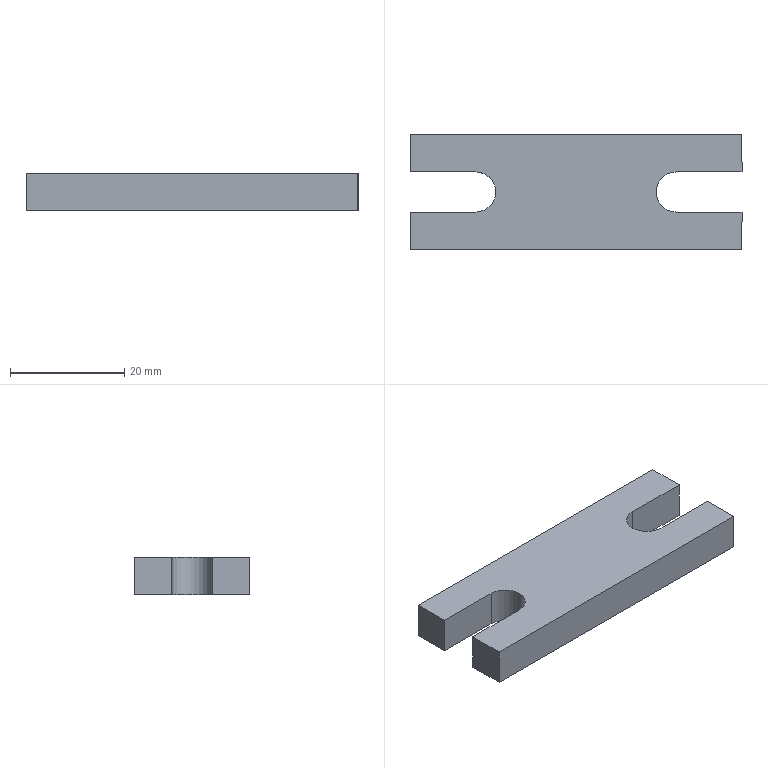Part | STEP file | 601-07-0071 | 1 solid | 15 faces | box 58 x 20 x 6.5 mm | volume 6243 mm3 | plane 12 | cylinder 3 | commonest cylinder face diameters 7 x3
STEP:
#1=CARTESIAN_POINT('',(0.,0.,0.));
#2=DIRECTION('',(0.,0.,1.));
#3=DIRECTION('',(1.,0.,0.));
#4=AXIS2_PLACEMENT_3D('',#1,#2,#3);
#5=CARTESIAN_POINT('',(-11.5,13.5,6.5));
#6=VERTEX_POINT('',#5);
#7=CARTESIAN_POINT('',(-11.5,13.5,0.));
#8=VERTEX_POINT('',#7);
#9=CARTESIAN_POINT('',(-11.5,13.5,6.5));
#10=DIRECTION('',(0.,0.,-1.));
#11=VECTOR('',#10,1.);
#12=LINE('',#9,#11);
#13=CARTESIAN_POINT('',(-11.5,10.,6.5));
#14=DIRECTION('',(0.,0.,-1.));
#15=DIRECTION('',(-1.,0.,0.));
#16=AXIS2_PLACEMENT_3D('',#13,#14,#15);
#17=CYLINDRICAL_SURFACE('',#16,3.5);
#18=CARTESIAN_POINT('',(1.571,0.));
#19=DIRECTION('',(0.,1.));
#20=VECTOR('',#19,1.);
#21=LINE('',#18,#20);
#22=(GEOMETRIC_REPRESENTATION_CONTEXT(2)PARAMETRIC_REPRESENTATION_CONTEXT()REPRESENTATION_CONTEXT('',''));
#23=DEFINITIONAL_REPRESENTATION('',(#21),#22);
#24=PCURVE('',#17,#23);
#25=CARTESIAN_POINT('',(-11.5,13.5,6.5));
#26=DIRECTION('',(0.,1.,0.));
#27=DIRECTION('',(0.,0.,1.));
#28=AXIS2_PLACEMENT_3D('',#25,#26,#27);
#29=PLANE('',#28);
#30=CARTESIAN_POINT('',(0.,0.));
#31=DIRECTION('',(-1.,0.));
#32=VECTOR('',#31,1.);
#33=LINE('',#30,#32);
#34=(GEOMETRIC_REPRESENTATION_CONTEXT(2)PARAMETRIC_REPRESENTATION_CONTEXT()REPRESENTATION_CONTEXT('',''));
#35=DEFINITIONAL_REPRESENTATION('',(#33),#34);
#36=PCURVE('',#29,#35);
#37=SURFACE_CURVE('',#12,(#24,#36),.PCURVE_S1.);
#38=EDGE_CURVE('',#6,#8,#37,.T.);
#39=ORIENTED_EDGE('',*,*,#38,.T.);
#40=CARTESIAN_POINT('',(-15.,10.,0.));
#41=VERTEX_POINT('',#40);
#42=CARTESIAN_POINT('',(-11.5,10.,0.));
#43=DIRECTION('',(0.,0.,-1.));
#44=DIRECTION('',(-1.,0.,0.));
#45=AXIS2_PLACEMENT_3D('',#42,#43,#44);
#46=CIRCLE('',#45,3.5);
#47=CARTESIAN_POINT('',(0.,6.5));
#48=DIRECTION('',(1.,0.));
#49=VECTOR('',#48,1.);
#50=LINE('',#47,#49);
#51=(GEOMETRIC_REPRESENTATION_CONTEXT(2)PARAMETRIC_REPRESENTATION_CONTEXT()REPRESENTATION_CONTEXT('',''));
#52=DEFINITIONAL_REPRESENTATION('',(#50),#51);
#53=PCURVE('',#17,#52);
#54=CARTESIAN_POINT('',(-11.5,10.,0.));
#55=DIRECTION('',(0.,0.,-1.));
#56=DIRECTION('',(-1.,0.,0.));
#57=AXIS2_PLACEMENT_3D('',#54,#55,#56);
#58=PLANE('',#57);
#59=CARTESIAN_POINT('',(0.,0.));
#60=DIRECTION('',(1.,0.));
#61=AXIS2_PLACEMENT_2D('',#59,#60);
#62=CIRCLE('',#61,3.5);
#63=(GEOMETRIC_REPRESENTATION_CONTEXT(2)PARAMETRIC_REPRESENTATION_CONTEXT()REPRESENTATION_CONTEXT('',''));
#64=DEFINITIONAL_REPRESENTATION('',(#62),#63);
#65=PCURVE('',#58,#64);
#66=SURFACE_CURVE('',#46,(#53,#65),.PCURVE_S1.);
#67=EDGE_CURVE('',#41,#8,#66,.T.);
#68=ORIENTED_EDGE('',*,*,#67,.F.);
#69=CARTESIAN_POINT('',(-15.,10.,6.5));
#70=VERTEX_POINT('',#69);
#71=CARTESIAN_POINT('',(-15.,10.,6.5));
#72=DIRECTION('',(0.,0.,-1.));
#73=VECTOR('',#72,1.);
#74=LINE('',#71,#73);
#75=CARTESIAN_POINT('',(0.,0.));
#76=DIRECTION('',(0.,1.));
#77=VECTOR('',#76,1.);
#78=LINE('',#75,#77);
#79=(GEOMETRIC_REPRESENTATION_CONTEXT(2)PARAMETRIC_REPRESENTATION_CONTEXT()REPRESENTATION_CONTEXT('',''));
#80=DEFINITIONAL_REPRESENTATION('',(#78),#79);
#81=PCURVE('',#17,#80);
#82=CARTESIAN_POINT('',(-11.5,10.,6.5));
#83=DIRECTION('',(0.,0.,-1.));
#84=DIRECTION('',(-1.,0.,0.));
#85=AXIS2_PLACEMENT_3D('',#82,#83,#84);
#86=CYLINDRICAL_SURFACE('',#85,3.5);
#87=CARTESIAN_POINT('',(6.283,0.));
#88=DIRECTION('',(0.,1.));
#89=VECTOR('',#88,1.);
#90=LINE('',#87,#89);
#91=(GEOMETRIC_REPRESENTATION_CONTEXT(2)PARAMETRIC_REPRESENTATION_CONTEXT()REPRESENTATION_CONTEXT('',''));
#92=DEFINITIONAL_REPRESENTATION('',(#90),#91);
#93=PCURVE('',#86,#92);
#94=SURFACE_CURVE('',#74,(#81,#93),.PCURVE_S1.);
#95=EDGE_CURVE('',#70,#41,#94,.T.);
#96=ORIENTED_EDGE('',*,*,#95,.F.);
#97=CARTESIAN_POINT('',(-11.5,10.,6.5));
#98=DIRECTION('',(0.,0.,-1.));
#99=DIRECTION('',(-1.,0.,0.));
#100=AXIS2_PLACEMENT_3D('',#97,#98,#99);
#101=CIRCLE('',#100,3.5);
#102=CARTESIAN_POINT('',(0.,0.));
#103=DIRECTION('',(1.,0.));
#104=VECTOR('',#103,1.);
#105=LINE('',#102,#104);
#106=(GEOMETRIC_REPRESENTATION_CONTEXT(2)PARAMETRIC_REPRESENTATION_CONTEXT()REPRESENTATION_CONTEXT('',''));
#107=DEFINITIONAL_REPRESENTATION('',(#105),#106);
#108=PCURVE('',#17,#107);
#109=CARTESIAN_POINT('',(-11.5,10.,6.5));
#110=DIRECTION('',(0.,0.,-1.));
#111=DIRECTION('',(-1.,0.,0.));
#112=AXIS2_PLACEMENT_3D('',#109,#110,#111);
#113=PLANE('',#112);
#114=CARTESIAN_POINT('',(0.,0.));
#115=DIRECTION('',(1.,0.));
#116=AXIS2_PLACEMENT_2D('',#114,#115);
#117=CIRCLE('',#116,3.5);
#118=(GEOMETRIC_REPRESENTATION_CONTEXT(2)PARAMETRIC_REPRESENTATION_CONTEXT()REPRESENTATION_CONTEXT('',''));
#119=DEFINITIONAL_REPRESENTATION('',(#117),#118);
#120=PCURVE('',#113,#119);
#121=SURFACE_CURVE('',#101,(#108,#120),.PCURVE_S1.);
#122=EDGE_CURVE('',#70,#6,#121,.T.);
#123=ORIENTED_EDGE('',*,*,#122,.T.);
#124=EDGE_LOOP('',(#39,#68,#96,#123));
#125=FACE_BOUND('',#124,.F.);
#126=ADVANCED_FACE('',(#125),#17,.F.);
#127=CARTESIAN_POINT('',(0.,0.,0.));
#128=VERTEX_POINT('',#127);
#129=CARTESIAN_POINT('',(0.,6.5,0.));
#130=VERTEX_POINT('',#129);
#131=CARTESIAN_POINT('',(0.,0.,0.));
#132=DIRECTION('',(0.,1.,0.));
#133=VECTOR('',#132,1.);
#134=LINE('',#131,#133);
#135=CARTESIAN_POINT('',(0.,0.,6.5));
#136=DIRECTION('',(-1.,0.,0.));
#137=DIRECTION('',(0.,-1.,0.));
#138=AXIS2_PLACEMENT_3D('',#135,#136,#137);
#139=PLANE('',#138);
#140=CARTESIAN_POINT('',(0.,-6.5));
#141=DIRECTION('',(-1.,0.));
#142=VECTOR('',#141,1.);
#143=LINE('',#140,#142);
#144=(GEOMETRIC_REPRESENTATION_CONTEXT(2)PARAMETRIC_REPRESENTATION_CONTEXT()REPRESENTATION_CONTEXT('',''));
#145=DEFINITIONAL_REPRESENTATION('',(#143),#144);
#146=PCURVE('',#139,#145);
#147=CARTESIAN_POINT('',(-11.5,-10.));
#148=DIRECTION('',(0.,1.));
#149=VECTOR('',#148,1.);
#150=LINE('',#147,#149);
#151=(GEOMETRIC_REPRESENTATION_CONTEXT(2)PARAMETRIC_REPRESENTATION_CONTEXT()REPRESENTATION_CONTEXT('',''));
#152=DEFINITIONAL_REPRESENTATION('',(#150),#151);
#153=PCURVE('',#58,#152);
#154=SURFACE_CURVE('',#134,(#146,#153),.PCURVE_S1.);
#155=EDGE_CURVE('',#128,#130,#154,.T.);
#156=ORIENTED_EDGE('',*,*,#155,.T.);
#157=CARTESIAN_POINT('',(0.,6.5,6.5));
#158=VERTEX_POINT('',#157);
#159=CARTESIAN_POINT('',(0.,6.5,6.5));
#160=DIRECTION('',(0.,0.,-1.));
#161=VECTOR('',#160,1.);
#162=LINE('',#159,#161);
#163=CARTESIAN_POINT('',(-6.5,0.));
#164=DIRECTION('',(0.,-1.));
#165=VECTOR('',#164,1.);
#166=LINE('',#163,#165);
#167=(GEOMETRIC_REPRESENTATION_CONTEXT(2)PARAMETRIC_REPRESENTATION_CONTEXT()REPRESENTATION_CONTEXT('',''));
#168=DEFINITIONAL_REPRESENTATION('',(#166),#167);
#169=PCURVE('',#139,#168);
#170=CARTESIAN_POINT('',(-11.5,6.5,6.5));
#171=DIRECTION('',(0.,-1.,0.));
#172=DIRECTION('',(0.,0.,-1.));
#173=AXIS2_PLACEMENT_3D('',#170,#171,#172);
#174=PLANE('',#173);
#175=CARTESIAN_POINT('',(0.,11.5));
#176=DIRECTION('',(1.,0.));
#177=VECTOR('',#176,1.);
#178=LINE('',#175,#177);
#179=(GEOMETRIC_REPRESENTATION_CONTEXT(2)PARAMETRIC_REPRESENTATION_CONTEXT()REPRESENTATION_CONTEXT('',''));
#180=DEFINITIONAL_REPRESENTATION('',(#178),#179);
#181=PCURVE('',#174,#180);
#182=SURFACE_CURVE('',#162,(#169,#181),.PCURVE_S1.);
#183=EDGE_CURVE('',#158,#130,#182,.T.);
#184=ORIENTED_EDGE('',*,*,#183,.F.);
#185=CARTESIAN_POINT('',(0.,0.,6.5));
#186=VERTEX_POINT('',#185);
#187=CARTESIAN_POINT('',(0.,0.,6.5));
#188=DIRECTION('',(0.,1.,0.));
#189=VECTOR('',#188,1.);
#190=LINE('',#187,#189);
#191=CARTESIAN_POINT('',(0.,0.));
#192=DIRECTION('',(-1.,0.));
#193=VECTOR('',#192,1.);
#194=LINE('',#191,#193);
#195=(GEOMETRIC_REPRESENTATION_CONTEXT(2)PARAMETRIC_REPRESENTATION_CONTEXT()REPRESENTATION_CONTEXT('',''));
#196=DEFINITIONAL_REPRESENTATION('',(#194),#195);
#197=PCURVE('',#139,#196);
#198=CARTESIAN_POINT('',(-11.5,-10.));
#199=DIRECTION('',(0.,1.));
#200=VECTOR('',#199,1.);
#201=LINE('',#198,#200);
#202=(GEOMETRIC_REPRESENTATION_CONTEXT(2)PARAMETRIC_REPRESENTATION_CONTEXT()REPRESENTATION_CONTEXT('',''));
#203=DEFINITIONAL_REPRESENTATION('',(#201),#202);
#204=PCURVE('',#113,#203);
#205=SURFACE_CURVE('',#190,(#197,#204),.PCURVE_S1.);
#206=EDGE_CURVE('',#186,#158,#205,.T.);
#207=ORIENTED_EDGE('',*,*,#206,.F.);
#208=CARTESIAN_POINT('',(0.,0.,6.5));
#209=DIRECTION('',(0.,0.,-1.));
#210=VECTOR('',#209,1.);
#211=LINE('',#208,#210);
#212=CARTESIAN_POINT('',(0.,0.));
#213=DIRECTION('',(0.,-1.));
#214=VECTOR('',#213,1.);
#215=LINE('',#212,#214);
#216=(GEOMETRIC_REPRESENTATION_CONTEXT(2)PARAMETRIC_REPRESENTATION_CONTEXT()REPRESENTATION_CONTEXT('',''));
#217=DEFINITIONAL_REPRESENTATION('',(#215),#216);
#218=PCURVE('',#139,#217);
#219=CARTESIAN_POINT('',(0.,0.,6.5));
#220=DIRECTION('',(0.,1.,0.));
#221=DIRECTION('',(-1.,0.,0.));
#222=AXIS2_PLACEMENT_3D('',#219,#220,#221);
#223=PLANE('',#222);
#224=CARTESIAN_POINT('',(0.,0.));
#225=DIRECTION('',(0.,-1.));
#226=VECTOR('',#225,1.);
#227=LINE('',#224,#226);
#228=(GEOMETRIC_REPRESENTATION_CONTEXT(2)PARAMETRIC_REPRESENTATION_CONTEXT()REPRESENTATION_CONTEXT('',''));
#229=DEFINITIONAL_REPRESENTATION('',(#227),#228);
#230=PCURVE('',#223,#229);
#231=SURFACE_CURVE('',#211,(#218,#230),.PCURVE_S1.);
#232=EDGE_CURVE('',#186,#128,#231,.T.);
#233=ORIENTED_EDGE('',*,*,#232,.T.);
#234=EDGE_LOOP('',(#156,#184,#207,#233));
#235=FACE_BOUND('',#234,.T.);
#236=ADVANCED_FACE('',(#235),#139,.F.);
#237=CARTESIAN_POINT('',(-11.5,6.5,0.));
#238=VERTEX_POINT('',#237);
#239=CARTESIAN_POINT('',(-11.5,6.5,0.));
#240=DIRECTION('',(-1.,0.,0.));
#241=VECTOR('',#240,1.);
#242=LINE('',#239,#241);
#243=CARTESIAN_POINT('',(6.5,0.));
#244=DIRECTION('',(0.,-1.));
#245=VECTOR('',#244,1.);
#246=LINE('',#243,#245);
#247=(GEOMETRIC_REPRESENTATION_CONTEXT(2)PARAMETRIC_REPRESENTATION_CONTEXT()REPRESENTATION_CONTEXT('',''));
#248=DEFINITIONAL_REPRESENTATION('',(#246),#247);
#249=PCURVE('',#174,#248);
#250=CARTESIAN_POINT('',(0.,-3.5));
#251=DIRECTION('',(1.,0.));
#252=VECTOR('',#251,1.);
#253=LINE('',#250,#252);
#254=(GEOMETRIC_REPRESENTATION_CONTEXT(2)PARAMETRIC_REPRESENTATION_CONTEXT()REPRESENTATION_CONTEXT('',''));
#255=DEFINITIONAL_REPRESENTATION('',(#253),#254);
#256=PCURVE('',#58,#255);
#257=SURFACE_CURVE('',#242,(#249,#256),.PCURVE_S1.);
#258=EDGE_CURVE('',#130,#238,#257,.T.);
#259=ORIENTED_EDGE('',*,*,#258,.T.);
#260=CARTESIAN_POINT('',(-11.5,6.5,6.5));
#261=VERTEX_POINT('',#260);
#262=CARTESIAN_POINT('',(-11.5,6.5,6.5));
#263=DIRECTION('',(0.,0.,-1.));
#264=VECTOR('',#263,1.);
#265=LINE('',#262,#264);
#266=CARTESIAN_POINT('',(0.,0.));
#267=DIRECTION('',(1.,0.));
#268=VECTOR('',#267,1.);
#269=LINE('',#266,#268);
#270=(GEOMETRIC_REPRESENTATION_CONTEXT(2)PARAMETRIC_REPRESENTATION_CONTEXT()REPRESENTATION_CONTEXT('',''));
#271=DEFINITIONAL_REPRESENTATION('',(#269),#270);
#272=PCURVE('',#174,#271);
#273=CARTESIAN_POINT('',(4.712,0.));
#274=DIRECTION('',(0.,1.));
#275=VECTOR('',#274,1.);
#276=LINE('',#273,#275);
#277=(GEOMETRIC_REPRESENTATION_CONTEXT(2)PARAMETRIC_REPRESENTATION_CONTEXT()REPRESENTATION_CONTEXT('',''));
#278=DEFINITIONAL_REPRESENTATION('',(#276),#277);
#279=PCURVE('',#86,#278);
#280=SURFACE_CURVE('',#265,(#272,#279),.PCURVE_S1.);
#281=EDGE_CURVE('',#261,#238,#280,.T.);
#282=ORIENTED_EDGE('',*,*,#281,.F.);
#283=CARTESIAN_POINT('',(-11.5,6.5,6.5));
#284=DIRECTION('',(-1.,0.,0.));
#285=VECTOR('',#284,1.);
#286=LINE('',#283,#285);
#287=CARTESIAN_POINT('',(0.,0.));
#288=DIRECTION('',(0.,-1.));
#289=VECTOR('',#288,1.);
#290=LINE('',#287,#289);
#291=(GEOMETRIC_REPRESENTATION_CONTEXT(2)PARAMETRIC_REPRESENTATION_CONTEXT()REPRESENTATION_CONTEXT('',''));
#292=DEFINITIONAL_REPRESENTATION('',(#290),#291);
#293=PCURVE('',#174,#292);
#294=CARTESIAN_POINT('',(0.,-3.5));
#295=DIRECTION('',(1.,0.));
#296=VECTOR('',#295,1.);
#297=LINE('',#294,#296);
#298=(GEOMETRIC_REPRESENTATION_CONTEXT(2)PARAMETRIC_REPRESENTATION_CONTEXT()REPRESENTATION_CONTEXT('',''));
#299=DEFINITIONAL_REPRESENTATION('',(#297),#298);
#300=PCURVE('',#113,#299);
#301=SURFACE_CURVE('',#286,(#293,#300),.PCURVE_S1.);
#302=EDGE_CURVE('',#158,#261,#301,.T.);
#303=ORIENTED_EDGE('',*,*,#302,.F.);
#304=ORIENTED_EDGE('',*,*,#183,.T.);
#305=EDGE_LOOP('',(#259,#282,#303,#304));
#306=FACE_BOUND('',#305,.T.);
#307=ADVANCED_FACE('',(#306),#174,.F.);
#308=CARTESIAN_POINT('',(-11.5,10.,0.));
#309=DIRECTION('',(0.,0.,-1.));
#310=DIRECTION('',(-1.,0.,0.));
#311=AXIS2_PLACEMENT_3D('',#308,#309,#310);
#312=CIRCLE('',#311,3.5);
#313=CARTESIAN_POINT('',(0.,6.5));
#314=DIRECTION('',(1.,0.));
#315=VECTOR('',#314,1.);
#316=LINE('',#313,#315);
#317=(GEOMETRIC_REPRESENTATION_CONTEXT(2)PARAMETRIC_REPRESENTATION_CONTEXT()REPRESENTATION_CONTEXT('',''));
#318=DEFINITIONAL_REPRESENTATION('',(#316),#317);
#319=PCURVE('',#86,#318);
#320=CARTESIAN_POINT('',(0.,0.));
#321=DIRECTION('',(1.,0.));
#322=AXIS2_PLACEMENT_2D('',#320,#321);
#323=CIRCLE('',#322,3.5);
#324=(GEOMETRIC_REPRESENTATION_CONTEXT(2)PARAMETRIC_REPRESENTATION_CONTEXT()REPRESENTATION_CONTEXT('',''));
#325=DEFINITIONAL_REPRESENTATION('',(#323),#324);
#326=PCURVE('',#58,#325);
#327=SURFACE_CURVE('',#312,(#319,#326),.PCURVE_S1.);
#328=EDGE_CURVE('',#238,#41,#327,.T.);
#329=ORIENTED_EDGE('',*,*,#328,.F.);
#330=ORIENTED_EDGE('',*,*,#281,.F.);
#331=CARTESIAN_POINT('',(-11.5,10.,6.5));
#332=DIRECTION('',(0.,0.,-1.));
#333=DIRECTION('',(-1.,0.,0.));
#334=AXIS2_PLACEMENT_3D('',#331,#332,#333);
#335=CIRCLE('',#334,3.5);
#336=CARTESIAN_POINT('',(0.,0.));
#337=DIRECTION('',(1.,0.));
#338=VECTOR('',#337,1.);
#339=LINE('',#336,#338);
#340=(GEOMETRIC_REPRESENTATION_CONTEXT(2)PARAMETRIC_REPRESENTATION_CONTEXT()REPRESENTATION_CONTEXT('',''));
#341=DEFINITIONAL_REPRESENTATION('',(#339),#340);
#342=PCURVE('',#86,#341);
#343=CARTESIAN_POINT('',(0.,0.));
#344=DIRECTION('',(1.,0.));
#345=AXIS2_PLACEMENT_2D('',#343,#344);
#346=CIRCLE('',#345,3.5);
#347=(GEOMETRIC_REPRESENTATION_CONTEXT(2)PARAMETRIC_REPRESENTATION_CONTEXT()REPRESENTATION_CONTEXT('',''));
#348=DEFINITIONAL_REPRESENTATION('',(#346),#347);
#349=PCURVE('',#113,#348);
#350=SURFACE_CURVE('',#335,(#342,#349),.PCURVE_S1.);
#351=EDGE_CURVE('',#261,#70,#350,.T.);
#352=ORIENTED_EDGE('',*,*,#351,.T.);
#353=ORIENTED_EDGE('',*,*,#95,.T.);
#354=EDGE_LOOP('',(#329,#330,#352,#353));
#355=FACE_BOUND('',#354,.F.);
#356=ADVANCED_FACE('',(#355),#86,.F.);
#357=CARTESIAN_POINT('',(0.,13.5,0.));
#358=VERTEX_POINT('',#357);
#359=CARTESIAN_POINT('',(-11.5,13.5,0.));
#360=DIRECTION('',(1.,0.,0.));
#361=VECTOR('',#360,1.);
#362=LINE('',#359,#361);
#363=CARTESIAN_POINT('',(-6.5,0.));
#364=DIRECTION('',(0.,1.));
#365=VECTOR('',#364,1.);
#366=LINE('',#363,#365);
#367=(GEOMETRIC_REPRESENTATION_CONTEXT(2)PARAMETRIC_REPRESENTATION_CONTEXT()REPRESENTATION_CONTEXT('',''));
#368=DEFINITIONAL_REPRESENTATION('',(#366),#367);
#369=PCURVE('',#29,#368);
#370=CARTESIAN_POINT('',(0.,3.5));
#371=DIRECTION('',(-1.,0.));
#372=VECTOR('',#371,1.);
#373=LINE('',#370,#372);
#374=(GEOMETRIC_REPRESENTATION_CONTEXT(2)PARAMETRIC_REPRESENTATION_CONTEXT()REPRESENTATION_CONTEXT('',''));
#375=DEFINITIONAL_REPRESENTATION('',(#373),#374);
#376=PCURVE('',#58,#375);
#377=SURFACE_CURVE('',#362,(#369,#376),.PCURVE_S1.);
#378=EDGE_CURVE('',#8,#358,#377,.T.);
#379=ORIENTED_EDGE('',*,*,#378,.T.);
#380=CARTESIAN_POINT('',(0.,13.5,6.5));
#381=VERTEX_POINT('',#380);
#382=CARTESIAN_POINT('',(0.,13.5,6.5));
#383=DIRECTION('',(0.,0.,-1.));
#384=VECTOR('',#383,1.);
#385=LINE('',#382,#384);
#386=CARTESIAN_POINT('',(0.,11.5));
#387=DIRECTION('',(-1.,0.));
#388=VECTOR('',#387,1.);
#389=LINE('',#386,#388);
#390=(GEOMETRIC_REPRESENTATION_CONTEXT(2)PARAMETRIC_REPRESENTATION_CONTEXT()REPRESENTATION_CONTEXT('',''));
#391=DEFINITIONAL_REPRESENTATION('',(#389),#390);
#392=PCURVE('',#29,#391);
#393=CARTESIAN_POINT('',(0.,13.5,6.5));
#394=DIRECTION('',(-1.,0.,0.));
#395=DIRECTION('',(0.,-1.,0.));
#396=AXIS2_PLACEMENT_3D('',#393,#394,#395);
#397=PLANE('',#396);
#398=CARTESIAN_POINT('',(0.,0.));
#399=DIRECTION('',(0.,-1.));
#400=VECTOR('',#399,1.);
#401=LINE('',#398,#400);
#402=(GEOMETRIC_REPRESENTATION_CONTEXT(2)PARAMETRIC_REPRESENTATION_CONTEXT()REPRESENTATION_CONTEXT('',''));
#403=DEFINITIONAL_REPRESENTATION('',(#401),#402);
#404=PCURVE('',#397,#403);
#405=SURFACE_CURVE('',#385,(#392,#404),.PCURVE_S1.);
#406=EDGE_CURVE('',#381,#358,#405,.T.);
#407=ORIENTED_EDGE('',*,*,#406,.F.);
#408=CARTESIAN_POINT('',(-11.5,13.5,6.5));
#409=DIRECTION('',(1.,0.,0.));
#410=VECTOR('',#409,1.);
#411=LINE('',#408,#410);
#412=CARTESIAN_POINT('',(0.,0.));
#413=DIRECTION('',(0.,1.));
#414=VECTOR('',#413,1.);
#415=LINE('',#412,#414);
#416=(GEOMETRIC_REPRESENTATION_CONTEXT(2)PARAMETRIC_REPRESENTATION_CONTEXT()REPRESENTATION_CONTEXT('',''));
#417=DEFINITIONAL_REPRESENTATION('',(#415),#416);
#418=PCURVE('',#29,#417);
#419=CARTESIAN_POINT('',(0.,3.5));
#420=DIRECTION('',(-1.,0.));
#421=VECTOR('',#420,1.);
#422=LINE('',#419,#421);
#423=(GEOMETRIC_REPRESENTATION_CONTEXT(2)PARAMETRIC_REPRESENTATION_CONTEXT()REPRESENTATION_CONTEXT('',''));
#424=DEFINITIONAL_REPRESENTATION('',(#422),#423);
#425=PCURVE('',#113,#424);
#426=SURFACE_CURVE('',#411,(#418,#425),.PCURVE_S1.);
#427=EDGE_CURVE('',#6,#381,#426,.T.);
#428=ORIENTED_EDGE('',*,*,#427,.F.);
#429=ORIENTED_EDGE('',*,*,#38,.T.);
#430=EDGE_LOOP('',(#379,#407,#428,#429));
#431=FACE_BOUND('',#430,.T.);
#432=ADVANCED_FACE('',(#431),#29,.F.);
#433=CARTESIAN_POINT('',(0.,20.,0.));
#434=VERTEX_POINT('',#433);
#435=CARTESIAN_POINT('',(0.,13.5,0.));
#436=DIRECTION('',(0.,1.,0.));
#437=VECTOR('',#436,1.);
#438=LINE('',#435,#437);
#439=CARTESIAN_POINT('',(0.,-6.5));
#440=DIRECTION('',(-1.,0.));
#441=VECTOR('',#440,1.);
#442=LINE('',#439,#441);
#443=(GEOMETRIC_REPRESENTATION_CONTEXT(2)PARAMETRIC_REPRESENTATION_CONTEXT()REPRESENTATION_CONTEXT('',''));
#444=DEFINITIONAL_REPRESENTATION('',(#442),#443);
#445=PCURVE('',#397,#444);
#446=CARTESIAN_POINT('',(-11.5,3.5));
#447=DIRECTION('',(0.,1.));
#448=VECTOR('',#447,1.);
#449=LINE('',#446,#448);
#450=(GEOMETRIC_REPRESENTATION_CONTEXT(2)PARAMETRIC_REPRESENTATION_CONTEXT()REPRESENTATION_CONTEXT('',''));
#451=DEFINITIONAL_REPRESENTATION('',(#449),#450);
#452=PCURVE('',#58,#451);
#453=SURFACE_CURVE('',#438,(#445,#452),.PCURVE_S1.);
#454=EDGE_CURVE('',#358,#434,#453,.T.);
#455=ORIENTED_EDGE('',*,*,#454,.T.);
#456=CARTESIAN_POINT('',(0.,20.,6.5));
#457=VERTEX_POINT('',#456);
#458=CARTESIAN_POINT('',(0.,20.,6.5));
#459=DIRECTION('',(0.,0.,-1.));
#460=VECTOR('',#459,1.);
#461=LINE('',#458,#460);
#462=CARTESIAN_POINT('',(-6.5,0.));
#463=DIRECTION('',(0.,-1.));
#464=VECTOR('',#463,1.);
#465=LINE('',#462,#464);
#466=(GEOMETRIC_REPRESENTATION_CONTEXT(2)PARAMETRIC_REPRESENTATION_CONTEXT()REPRESENTATION_CONTEXT('',''));
#467=DEFINITIONAL_REPRESENTATION('',(#465),#466);
#468=PCURVE('',#397,#467);
#469=CARTESIAN_POINT('',(0.,20.,6.5));
#470=DIRECTION('',(0.,-1.,0.));
#471=DIRECTION('',(1.,0.,0.));
#472=AXIS2_PLACEMENT_3D('',#469,#470,#471);
#473=PLANE('',#472);
#474=CARTESIAN_POINT('',(0.,0.));
#475=DIRECTION('',(0.,-1.));
#476=VECTOR('',#475,1.);
#477=LINE('',#474,#476);
#478=(GEOMETRIC_REPRESENTATION_CONTEXT(2)PARAMETRIC_REPRESENTATION_CONTEXT()REPRESENTATION_CONTEXT('',''));
#479=DEFINITIONAL_REPRESENTATION('',(#477),#478);
#480=PCURVE('',#473,#479);
#481=SURFACE_CURVE('',#461,(#468,#480),.PCURVE_S1.);
#482=EDGE_CURVE('',#457,#434,#481,.T.);
#483=ORIENTED_EDGE('',*,*,#482,.F.);
#484=CARTESIAN_POINT('',(0.,13.5,6.5));
#485=DIRECTION('',(0.,1.,0.));
#486=VECTOR('',#485,1.);
#487=LINE('',#484,#486);
#488=CARTESIAN_POINT('',(0.,0.));
#489=DIRECTION('',(-1.,0.));
#490=VECTOR('',#489,1.);
#491=LINE('',#488,#490);
#492=(GEOMETRIC_REPRESENTATION_CONTEXT(2)PARAMETRIC_REPRESENTATION_CONTEXT()REPRESENTATION_CONTEXT('',''));
#493=DEFINITIONAL_REPRESENTATION('',(#491),#492);
#494=PCURVE('',#397,#493);
#495=CARTESIAN_POINT('',(-11.5,3.5));
#496=DIRECTION('',(0.,1.));
#497=VECTOR('',#496,1.);
#498=LINE('',#495,#497);
#499=(GEOMETRIC_REPRESENTATION_CONTEXT(2)PARAMETRIC_REPRESENTATION_CONTEXT()REPRESENTATION_CONTEXT('',''));
#500=DEFINITIONAL_REPRESENTATION('',(#498),#499);
#501=PCURVE('',#113,#500);
#502=SURFACE_CURVE('',#487,(#494,#501),.PCURVE_S1.);
#503=EDGE_CURVE('',#381,#457,#502,.T.);
#504=ORIENTED_EDGE('',*,*,#503,.F.);
#505=ORIENTED_EDGE('',*,*,#406,.T.);
#506=EDGE_LOOP('',(#455,#483,#504,#505));
#507=FACE_BOUND('',#506,.T.);
#508=ADVANCED_FACE('',(#507),#397,.F.);
#509=CARTESIAN_POINT('',(-58.,20.,0.));
#510=VERTEX_POINT('',#509);
#511=CARTESIAN_POINT('',(0.,20.,0.));
#512=DIRECTION('',(-1.,0.,0.));
#513=VECTOR('',#512,1.);
#514=LINE('',#511,#513);
#515=CARTESIAN_POINT('',(0.,-6.5));
#516=DIRECTION('',(-1.,0.));
#517=VECTOR('',#516,1.);
#518=LINE('',#515,#517);
#519=(GEOMETRIC_REPRESENTATION_CONTEXT(2)PARAMETRIC_REPRESENTATION_CONTEXT()REPRESENTATION_CONTEXT('',''));
#520=DEFINITIONAL_REPRESENTATION('',(#518),#519);
#521=PCURVE('',#473,#520);
#522=CARTESIAN_POINT('',(-11.5,10.));
#523=DIRECTION('',(1.,0.));
#524=VECTOR('',#523,1.);
#525=LINE('',#522,#524);
#526=(GEOMETRIC_REPRESENTATION_CONTEXT(2)PARAMETRIC_REPRESENTATION_CONTEXT()REPRESENTATION_CONTEXT('',''));
#527=DEFINITIONAL_REPRESENTATION('',(#525),#526);
#528=PCURVE('',#58,#527);
#529=SURFACE_CURVE('',#514,(#521,#528),.PCURVE_S1.);
#530=EDGE_CURVE('',#434,#510,#529,.T.);
#531=ORIENTED_EDGE('',*,*,#530,.T.);
#532=CARTESIAN_POINT('',(-58.,20.,6.5));
#533=VERTEX_POINT('',#532);
#534=CARTESIAN_POINT('',(-58.,20.,6.5));
#535=DIRECTION('',(0.,0.,-1.));
#536=VECTOR('',#535,1.);
#537=LINE('',#534,#536);
#538=CARTESIAN_POINT('',(-58.,0.));
#539=DIRECTION('',(0.,-1.));
#540=VECTOR('',#539,1.);
#541=LINE('',#538,#540);
#542=(GEOMETRIC_REPRESENTATION_CONTEXT(2)PARAMETRIC_REPRESENTATION_CONTEXT()REPRESENTATION_CONTEXT('',''));
#543=DEFINITIONAL_REPRESENTATION('',(#541),#542);
#544=PCURVE('',#473,#543);
#545=CARTESIAN_POINT('',(-58.,13.5,6.5));
#546=DIRECTION('',(1.,0.,0.));
#547=DIRECTION('',(0.,0.,-1.));
#548=AXIS2_PLACEMENT_3D('',#545,#546,#547);
#549=PLANE('',#548);
#550=CARTESIAN_POINT('',(0.,6.5));
#551=DIRECTION('',(1.,0.));
#552=VECTOR('',#551,1.);
#553=LINE('',#550,#552);
#554=(GEOMETRIC_REPRESENTATION_CONTEXT(2)PARAMETRIC_REPRESENTATION_CONTEXT()REPRESENTATION_CONTEXT('',''));
#555=DEFINITIONAL_REPRESENTATION('',(#553),#554);
#556=PCURVE('',#549,#555);
#557=SURFACE_CURVE('',#537,(#544,#556),.PCURVE_S1.);
#558=EDGE_CURVE('',#533,#510,#557,.T.);
#559=ORIENTED_EDGE('',*,*,#558,.F.);
#560=CARTESIAN_POINT('',(0.,20.,6.5));
#561=DIRECTION('',(-1.,0.,0.));
#562=VECTOR('',#561,1.);
#563=LINE('',#560,#562);
#564=CARTESIAN_POINT('',(0.,0.));
#565=DIRECTION('',(-1.,0.));
#566=VECTOR('',#565,1.);
#567=LINE('',#564,#566);
#568=(GEOMETRIC_REPRESENTATION_CONTEXT(2)PARAMETRIC_REPRESENTATION_CONTEXT()REPRESENTATION_CONTEXT('',''));
#569=DEFINITIONAL_REPRESENTATION('',(#567),#568);
#570=PCURVE('',#473,#569);
#571=CARTESIAN_POINT('',(-11.5,10.));
#572=DIRECTION('',(1.,0.));
#573=VECTOR('',#572,1.);
#574=LINE('',#571,#573);
#575=(GEOMETRIC_REPRESENTATION_CONTEXT(2)PARAMETRIC_REPRESENTATION_CONTEXT()REPRESENTATION_CONTEXT('',''));
#576=DEFINITIONAL_REPRESENTATION('',(#574),#575);
#577=PCURVE('',#113,#576);
#578=SURFACE_CURVE('',#563,(#570,#577),.PCURVE_S1.);
#579=EDGE_CURVE('',#457,#533,#578,.T.);
#580=ORIENTED_EDGE('',*,*,#579,.F.);
#581=ORIENTED_EDGE('',*,*,#482,.T.);
#582=EDGE_LOOP('',(#531,#559,#580,#581));
#583=FACE_BOUND('',#582,.T.);
#584=ADVANCED_FACE('',(#583),#473,.F.);
#585=CARTESIAN_POINT('',(-58.,13.5,0.));
#586=VERTEX_POINT('',#585);
#587=CARTESIAN_POINT('',(-58.,13.5,0.));
#588=DIRECTION('',(0.,-1.,0.));
#589=VECTOR('',#588,1.);
#590=LINE('',#587,#589);
#591=CARTESIAN_POINT('',(6.5,0.));
#592=DIRECTION('',(0.,-1.));
#593=VECTOR('',#592,1.);
#594=LINE('',#591,#593);
#595=(GEOMETRIC_REPRESENTATION_CONTEXT(2)PARAMETRIC_REPRESENTATION_CONTEXT()REPRESENTATION_CONTEXT('',''));
#596=DEFINITIONAL_REPRESENTATION('',(#594),#595);
#597=PCURVE('',#549,#596);
#598=CARTESIAN_POINT('',(46.5,3.5));
#599=DIRECTION('',(0.,-1.));
#600=VECTOR('',#599,1.);
#601=LINE('',#598,#600);
#602=(GEOMETRIC_REPRESENTATION_CONTEXT(2)PARAMETRIC_REPRESENTATION_CONTEXT()REPRESENTATION_CONTEXT('',''));
#603=DEFINITIONAL_REPRESENTATION('',(#601),#602);
#604=PCURVE('',#58,#603);
#605=SURFACE_CURVE('',#590,(#597,#604),.PCURVE_S1.);
#606=EDGE_CURVE('',#510,#586,#605,.T.);
#607=ORIENTED_EDGE('',*,*,#606,.T.);
#608=CARTESIAN_POINT('',(-58.,13.5,6.5));
#609=VERTEX_POINT('',#608);
#610=CARTESIAN_POINT('',(-58.,13.5,6.5));
#611=DIRECTION('',(0.,0.,-1.));
#612=VECTOR('',#611,1.);
#613=LINE('',#610,#612);
#614=CARTESIAN_POINT('',(0.,0.));
#615=DIRECTION('',(1.,0.));
#616=VECTOR('',#615,1.);
#617=LINE('',#614,#616);
#618=(GEOMETRIC_REPRESENTATION_CONTEXT(2)PARAMETRIC_REPRESENTATION_CONTEXT()REPRESENTATION_CONTEXT('',''));
#619=DEFINITIONAL_REPRESENTATION('',(#617),#618);
#620=PCURVE('',#549,#619);
#621=CARTESIAN_POINT('',(-46.5,13.5,6.5));
#622=DIRECTION('',(0.,1.,0.));
#623=DIRECTION('',(0.,0.,1.));
#624=AXIS2_PLACEMENT_3D('',#621,#622,#623);
#625=PLANE('',#624);
#626=CARTESIAN_POINT('',(0.,-11.5));
#627=DIRECTION('',(-1.,0.));
#628=VECTOR('',#627,1.);
#629=LINE('',#626,#628);
#630=(GEOMETRIC_REPRESENTATION_CONTEXT(2)PARAMETRIC_REPRESENTATION_CONTEXT()REPRESENTATION_CONTEXT('',''));
#631=DEFINITIONAL_REPRESENTATION('',(#629),#630);
#632=PCURVE('',#625,#631);
#633=SURFACE_CURVE('',#613,(#620,#632),.PCURVE_S1.);
#634=EDGE_CURVE('',#609,#586,#633,.T.);
#635=ORIENTED_EDGE('',*,*,#634,.F.);
#636=CARTESIAN_POINT('',(-58.,13.5,6.5));
#637=DIRECTION('',(0.,-1.,0.));
#638=VECTOR('',#637,1.);
#639=LINE('',#636,#638);
#640=CARTESIAN_POINT('',(0.,0.));
#641=DIRECTION('',(0.,-1.));
#642=VECTOR('',#641,1.);
#643=LINE('',#640,#642);
#644=(GEOMETRIC_REPRESENTATION_CONTEXT(2)PARAMETRIC_REPRESENTATION_CONTEXT()REPRESENTATION_CONTEXT('',''));
#645=DEFINITIONAL_REPRESENTATION('',(#643),#644);
#646=PCURVE('',#549,#645);
#647=CARTESIAN_POINT('',(46.5,3.5));
#648=DIRECTION('',(0.,-1.));
#649=VECTOR('',#648,1.);
#650=LINE('',#647,#649);
#651=(GEOMETRIC_REPRESENTATION_CONTEXT(2)PARAMETRIC_REPRESENTATION_CONTEXT()REPRESENTATION_CONTEXT('',''));
#652=DEFINITIONAL_REPRESENTATION('',(#650),#651);
#653=PCURVE('',#113,#652);
#654=SURFACE_CURVE('',#639,(#646,#653),.PCURVE_S1.);
#655=EDGE_CURVE('',#533,#609,#654,.T.);
#656=ORIENTED_EDGE('',*,*,#655,.F.);
#657=ORIENTED_EDGE('',*,*,#558,.T.);
#658=EDGE_LOOP('',(#607,#635,#656,#657));
#659=FACE_BOUND('',#658,.T.);
#660=ADVANCED_FACE('',(#659),#549,.F.);
#661=CARTESIAN_POINT('',(-46.5,13.5,0.));
#662=VERTEX_POINT('',#661);
#663=CARTESIAN_POINT('',(-46.5,13.5,0.));
#664=DIRECTION('',(1.,0.,0.));
#665=VECTOR('',#664,1.);
#666=LINE('',#663,#665);
#667=CARTESIAN_POINT('',(-6.5,0.));
#668=DIRECTION('',(0.,1.));
#669=VECTOR('',#668,1.);
#670=LINE('',#667,#669);
#671=(GEOMETRIC_REPRESENTATION_CONTEXT(2)PARAMETRIC_REPRESENTATION_CONTEXT()REPRESENTATION_CONTEXT('',''));
#672=DEFINITIONAL_REPRESENTATION('',(#670),#671);
#673=PCURVE('',#625,#672);
#674=CARTESIAN_POINT('',(35.,3.5));
#675=DIRECTION('',(-1.,0.));
#676=VECTOR('',#675,1.);
#677=LINE('',#674,#676);
#678=(GEOMETRIC_REPRESENTATION_CONTEXT(2)PARAMETRIC_REPRESENTATION_CONTEXT()REPRESENTATION_CONTEXT('',''));
#679=DEFINITIONAL_REPRESENTATION('',(#677),#678);
#680=PCURVE('',#58,#679);
#681=SURFACE_CURVE('',#666,(#673,#680),.PCURVE_S1.);
#682=EDGE_CURVE('',#586,#662,#681,.T.);
#683=ORIENTED_EDGE('',*,*,#682,.T.);
#684=CARTESIAN_POINT('',(-46.5,13.5,6.5));
#685=VERTEX_POINT('',#684);
#686=CARTESIAN_POINT('',(-46.5,13.5,6.5));
#687=DIRECTION('',(0.,0.,-1.));
#688=VECTOR('',#687,1.);
#689=LINE('',#686,#688);
#690=CARTESIAN_POINT('',(0.,0.));
#691=DIRECTION('',(-1.,0.));
#692=VECTOR('',#691,1.);
#693=LINE('',#690,#692);
#694=(GEOMETRIC_REPRESENTATION_CONTEXT(2)PARAMETRIC_REPRESENTATION_CONTEXT()REPRESENTATION_CONTEXT('',''));
#695=DEFINITIONAL_REPRESENTATION('',(#693),#694);
#696=PCURVE('',#625,#695);
#697=CARTESIAN_POINT('',(-46.5,10.,6.5));
#698=DIRECTION('',(0.,0.,-1.));
#699=DIRECTION('',(-1.,0.,0.));
#700=AXIS2_PLACEMENT_3D('',#697,#698,#699);
#701=CYLINDRICAL_SURFACE('',#700,3.5);
#702=CARTESIAN_POINT('',(1.571,0.));
#703=DIRECTION('',(0.,1.));
#704=VECTOR('',#703,1.);
#705=LINE('',#702,#704);
#706=(GEOMETRIC_REPRESENTATION_CONTEXT(2)PARAMETRIC_REPRESENTATION_CONTEXT()REPRESENTATION_CONTEXT('',''));
#707=DEFINITIONAL_REPRESENTATION('',(#705),#706);
#708=PCURVE('',#701,#707);
#709=SURFACE_CURVE('',#689,(#696,#708),.PCURVE_S1.);
#710=EDGE_CURVE('',#685,#662,#709,.T.);
#711=ORIENTED_EDGE('',*,*,#710,.F.);
#712=CARTESIAN_POINT('',(-46.5,13.5,6.5));
#713=DIRECTION('',(1.,0.,0.));
#714=VECTOR('',#713,1.);
#715=LINE('',#712,#714);
#716=CARTESIAN_POINT('',(0.,0.));
#717=DIRECTION('',(0.,1.));
#718=VECTOR('',#717,1.);
#719=LINE('',#716,#718);
#720=(GEOMETRIC_REPRESENTATION_CONTEXT(2)PARAMETRIC_REPRESENTATION_CONTEXT()REPRESENTATION_CONTEXT('',''));
#721=DEFINITIONAL_REPRESENTATION('',(#719),#720);
#722=PCURVE('',#625,#721);
#723=CARTESIAN_POINT('',(35.,3.5));
#724=DIRECTION('',(-1.,0.));
#725=VECTOR('',#724,1.);
#726=LINE('',#723,#725);
#727=(GEOMETRIC_REPRESENTATION_CONTEXT(2)PARAMETRIC_REPRESENTATION_CONTEXT()REPRESENTATION_CONTEXT('',''));
#728=DEFINITIONAL_REPRESENTATION('',(#726),#727);
#729=PCURVE('',#113,#728);
#730=SURFACE_CURVE('',#715,(#722,#729),.PCURVE_S1.);
#731=EDGE_CURVE('',#609,#685,#730,.T.);
#732=ORIENTED_EDGE('',*,*,#731,.F.);
#733=ORIENTED_EDGE('',*,*,#634,.T.);
#734=EDGE_LOOP('',(#683,#711,#732,#733));
#735=FACE_BOUND('',#734,.T.);
#736=ADVANCED_FACE('',(#735),#625,.F.);
#737=ORIENTED_EDGE('',*,*,#710,.F.);
#738=CARTESIAN_POINT('',(-46.5,6.5,6.5));
#739=VERTEX_POINT('',#738);
#740=CARTESIAN_POINT('',(-46.5,10.,6.5));
#741=DIRECTION('',(0.,0.,-1.));
#742=DIRECTION('',(1.,0.,0.));
#743=AXIS2_PLACEMENT_3D('',#740,#741,#742);
#744=CIRCLE('',#743,3.5);
#745=CARTESIAN_POINT('',(-3.142,0.));
#746=DIRECTION('',(1.,0.));
#747=VECTOR('',#746,1.);
#748=LINE('',#745,#747);
#749=(GEOMETRIC_REPRESENTATION_CONTEXT(2)PARAMETRIC_REPRESENTATION_CONTEXT()REPRESENTATION_CONTEXT('',''));
#750=DEFINITIONAL_REPRESENTATION('',(#748),#749);
#751=PCURVE('',#701,#750);
#752=CARTESIAN_POINT('',(35.,0.));
#753=DIRECTION('',(-1.,0.));
#754=AXIS2_PLACEMENT_2D('',#752,#753);
#755=CIRCLE('',#754,3.5);
#756=(GEOMETRIC_REPRESENTATION_CONTEXT(2)PARAMETRIC_REPRESENTATION_CONTEXT()REPRESENTATION_CONTEXT('',''));
#757=DEFINITIONAL_REPRESENTATION('',(#755),#756);
#758=PCURVE('',#113,#757);
#759=SURFACE_CURVE('',#744,(#751,#758),.PCURVE_S1.);
#760=EDGE_CURVE('',#685,#739,#759,.T.);
#761=ORIENTED_EDGE('',*,*,#760,.T.);
#762=CARTESIAN_POINT('',(-46.5,6.5,0.));
#763=VERTEX_POINT('',#762);
#764=CARTESIAN_POINT('',(-46.5,6.5,6.5));
#765=DIRECTION('',(0.,0.,-1.));
#766=VECTOR('',#765,1.);
#767=LINE('',#764,#766);
#768=CARTESIAN_POINT('',(4.712,0.));
#769=DIRECTION('',(0.,1.));
#770=VECTOR('',#769,1.);
#771=LINE('',#768,#770);
#772=(GEOMETRIC_REPRESENTATION_CONTEXT(2)PARAMETRIC_REPRESENTATION_CONTEXT()REPRESENTATION_CONTEXT('',''));
#773=DEFINITIONAL_REPRESENTATION('',(#771),#772);
#774=PCURVE('',#701,#773);
#775=CARTESIAN_POINT('',(-46.5,6.5,6.5));
#776=DIRECTION('',(0.,-1.,0.));
#777=DIRECTION('',(0.,0.,-1.));
#778=AXIS2_PLACEMENT_3D('',#775,#776,#777);
#779=PLANE('',#778);
#780=CARTESIAN_POINT('',(0.,0.));
#781=DIRECTION('',(1.,0.));
#782=VECTOR('',#781,1.);
#783=LINE('',#780,#782);
#784=(GEOMETRIC_REPRESENTATION_CONTEXT(2)PARAMETRIC_REPRESENTATION_CONTEXT()REPRESENTATION_CONTEXT('',''));
#785=DEFINITIONAL_REPRESENTATION('',(#783),#784);
#786=PCURVE('',#779,#785);
#787=SURFACE_CURVE('',#767,(#774,#786),.PCURVE_S1.);
#788=EDGE_CURVE('',#739,#763,#787,.T.);
#789=ORIENTED_EDGE('',*,*,#788,.T.);
#790=CARTESIAN_POINT('',(-46.5,10.,0.));
#791=DIRECTION('',(0.,0.,-1.));
#792=DIRECTION('',(1.,0.,0.));
#793=AXIS2_PLACEMENT_3D('',#790,#791,#792);
#794=CIRCLE('',#793,3.5);
#795=CARTESIAN_POINT('',(-3.142,6.5));
#796=DIRECTION('',(1.,0.));
#797=VECTOR('',#796,1.);
#798=LINE('',#795,#797);
#799=(GEOMETRIC_REPRESENTATION_CONTEXT(2)PARAMETRIC_REPRESENTATION_CONTEXT()REPRESENTATION_CONTEXT('',''));
#800=DEFINITIONAL_REPRESENTATION('',(#798),#799);
#801=PCURVE('',#701,#800);
#802=CARTESIAN_POINT('',(35.,0.));
#803=DIRECTION('',(-1.,0.));
#804=AXIS2_PLACEMENT_2D('',#802,#803);
#805=CIRCLE('',#804,3.5);
#806=(GEOMETRIC_REPRESENTATION_CONTEXT(2)PARAMETRIC_REPRESENTATION_CONTEXT()REPRESENTATION_CONTEXT('',''));
#807=DEFINITIONAL_REPRESENTATION('',(#805),#806);
#808=PCURVE('',#58,#807);
#809=SURFACE_CURVE('',#794,(#801,#808),.PCURVE_S1.);
#810=EDGE_CURVE('',#662,#763,#809,.T.);
#811=ORIENTED_EDGE('',*,*,#810,.F.);
#812=EDGE_LOOP('',(#737,#761,#789,#811));
#813=FACE_BOUND('',#812,.F.);
#814=ADVANCED_FACE('',(#813),#701,.F.);
#815=CARTESIAN_POINT('',(-58.,6.5,0.));
#816=VERTEX_POINT('',#815);
#817=CARTESIAN_POINT('',(-46.5,6.5,0.));
#818=DIRECTION('',(-1.,0.,0.));
#819=VECTOR('',#818,1.);
#820=LINE('',#817,#819);
#821=CARTESIAN_POINT('',(6.5,0.));
#822=DIRECTION('',(0.,-1.));
#823=VECTOR('',#822,1.);
#824=LINE('',#821,#823);
#825=(GEOMETRIC_REPRESENTATION_CONTEXT(2)PARAMETRIC_REPRESENTATION_CONTEXT()REPRESENTATION_CONTEXT('',''));
#826=DEFINITIONAL_REPRESENTATION('',(#824),#825);
#827=PCURVE('',#779,#826);
#828=CARTESIAN_POINT('',(35.,-3.5));
#829=DIRECTION('',(1.,0.));
#830=VECTOR('',#829,1.);
#831=LINE('',#828,#830);
#832=(GEOMETRIC_REPRESENTATION_CONTEXT(2)PARAMETRIC_REPRESENTATION_CONTEXT()REPRESENTATION_CONTEXT('',''));
#833=DEFINITIONAL_REPRESENTATION('',(#831),#832);
#834=PCURVE('',#58,#833);
#835=SURFACE_CURVE('',#820,(#827,#834),.PCURVE_S1.);
#836=EDGE_CURVE('',#763,#816,#835,.T.);
#837=ORIENTED_EDGE('',*,*,#836,.T.);
#838=CARTESIAN_POINT('',(-58.,6.5,6.5));
#839=VERTEX_POINT('',#838);
#840=CARTESIAN_POINT('',(-58.,6.5,6.5));
#841=DIRECTION('',(0.,0.,-1.));
#842=VECTOR('',#841,1.);
#843=LINE('',#840,#842);
#844=CARTESIAN_POINT('',(0.,-11.5));
#845=DIRECTION('',(1.,0.));
#846=VECTOR('',#845,1.);
#847=LINE('',#844,#846);
#848=(GEOMETRIC_REPRESENTATION_CONTEXT(2)PARAMETRIC_REPRESENTATION_CONTEXT()REPRESENTATION_CONTEXT('',''));
#849=DEFINITIONAL_REPRESENTATION('',(#847),#848);
#850=PCURVE('',#779,#849);
#851=CARTESIAN_POINT('',(-58.,0.,6.5));
#852=DIRECTION('',(1.,0.,0.));
#853=DIRECTION('',(0.,0.,-1.));
#854=AXIS2_PLACEMENT_3D('',#851,#852,#853);
#855=PLANE('',#854);
#856=CARTESIAN_POINT('',(0.,6.5));
#857=DIRECTION('',(1.,0.));
#858=VECTOR('',#857,1.);
#859=LINE('',#856,#858);
#860=(GEOMETRIC_REPRESENTATION_CONTEXT(2)PARAMETRIC_REPRESENTATION_CONTEXT()REPRESENTATION_CONTEXT('',''));
#861=DEFINITIONAL_REPRESENTATION('',(#859),#860);
#862=PCURVE('',#855,#861);
#863=SURFACE_CURVE('',#843,(#850,#862),.PCURVE_S1.);
#864=EDGE_CURVE('',#839,#816,#863,.T.);
#865=ORIENTED_EDGE('',*,*,#864,.F.);
#866=CARTESIAN_POINT('',(-46.5,6.5,6.5));
#867=DIRECTION('',(-1.,0.,0.));
#868=VECTOR('',#867,1.);
#869=LINE('',#866,#868);
#870=CARTESIAN_POINT('',(0.,0.));
#871=DIRECTION('',(0.,-1.));
#872=VECTOR('',#871,1.);
#873=LINE('',#870,#872);
#874=(GEOMETRIC_REPRESENTATION_CONTEXT(2)PARAMETRIC_REPRESENTATION_CONTEXT()REPRESENTATION_CONTEXT('',''));
#875=DEFINITIONAL_REPRESENTATION('',(#873),#874);
#876=PCURVE('',#779,#875);
#877=CARTESIAN_POINT('',(35.,-3.5));
#878=DIRECTION('',(1.,0.));
#879=VECTOR('',#878,1.);
#880=LINE('',#877,#879);
#881=(GEOMETRIC_REPRESENTATION_CONTEXT(2)PARAMETRIC_REPRESENTATION_CONTEXT()REPRESENTATION_CONTEXT('',''));
#882=DEFINITIONAL_REPRESENTATION('',(#880),#881);
#883=PCURVE('',#113,#882);
#884=SURFACE_CURVE('',#869,(#876,#883),.PCURVE_S1.);
#885=EDGE_CURVE('',#739,#839,#884,.T.);
#886=ORIENTED_EDGE('',*,*,#885,.F.);
#887=ORIENTED_EDGE('',*,*,#788,.T.);
#888=EDGE_LOOP('',(#837,#865,#886,#887));
#889=FACE_BOUND('',#888,.T.);
#890=ADVANCED_FACE('',(#889),#779,.F.);
#891=CARTESIAN_POINT('',(-58.,0.,0.));
#892=VERTEX_POINT('',#891);
#893=CARTESIAN_POINT('',(-58.,0.,0.));
#894=DIRECTION('',(0.,-1.,0.));
#895=VECTOR('',#894,1.);
#896=LINE('',#893,#895);
#897=CARTESIAN_POINT('',(6.5,0.));
#898=DIRECTION('',(0.,-1.));
#899=VECTOR('',#898,1.);
#900=LINE('',#897,#899);
#901=(GEOMETRIC_REPRESENTATION_CONTEXT(2)PARAMETRIC_REPRESENTATION_CONTEXT()REPRESENTATION_CONTEXT('',''));
#902=DEFINITIONAL_REPRESENTATION('',(#900),#901);
#903=PCURVE('',#855,#902);
#904=CARTESIAN_POINT('',(46.5,-10.));
#905=DIRECTION('',(0.,-1.));
#906=VECTOR('',#905,1.);
#907=LINE('',#904,#906);
#908=(GEOMETRIC_REPRESENTATION_CONTEXT(2)PARAMETRIC_REPRESENTATION_CONTEXT()REPRESENTATION_CONTEXT('',''));
#909=DEFINITIONAL_REPRESENTATION('',(#907),#908);
#910=PCURVE('',#58,#909);
#911=SURFACE_CURVE('',#896,(#903,#910),.PCURVE_S1.);
#912=EDGE_CURVE('',#816,#892,#911,.T.);
#913=ORIENTED_EDGE('',*,*,#912,.T.);
#914=CARTESIAN_POINT('',(-58.,0.,6.5));
#915=VERTEX_POINT('',#914);
#916=CARTESIAN_POINT('',(-58.,0.,6.5));
#917=DIRECTION('',(0.,0.,-1.));
#918=VECTOR('',#917,1.);
#919=LINE('',#916,#918);
#920=CARTESIAN_POINT('',(0.,0.));
#921=DIRECTION('',(1.,0.));
#922=VECTOR('',#921,1.);
#923=LINE('',#920,#922);
#924=(GEOMETRIC_REPRESENTATION_CONTEXT(2)PARAMETRIC_REPRESENTATION_CONTEXT()REPRESENTATION_CONTEXT('',''));
#925=DEFINITIONAL_REPRESENTATION('',(#923),#924);
#926=PCURVE('',#855,#925);
#927=CARTESIAN_POINT('',(58.,0.));
#928=DIRECTION('',(0.,-1.));
#929=VECTOR('',#928,1.);
#930=LINE('',#927,#929);
#931=(GEOMETRIC_REPRESENTATION_CONTEXT(2)PARAMETRIC_REPRESENTATION_CONTEXT()REPRESENTATION_CONTEXT('',''));
#932=DEFINITIONAL_REPRESENTATION('',(#930),#931);
#933=PCURVE('',#223,#932);
#934=SURFACE_CURVE('',#919,(#926,#933),.PCURVE_S1.);
#935=EDGE_CURVE('',#915,#892,#934,.T.);
#936=ORIENTED_EDGE('',*,*,#935,.F.);
#937=CARTESIAN_POINT('',(-58.,0.,6.5));
#938=DIRECTION('',(0.,-1.,0.));
#939=VECTOR('',#938,1.);
#940=LINE('',#937,#939);
#941=CARTESIAN_POINT('',(0.,0.));
#942=DIRECTION('',(0.,-1.));
#943=VECTOR('',#942,1.);
#944=LINE('',#941,#943);
#945=(GEOMETRIC_REPRESENTATION_CONTEXT(2)PARAMETRIC_REPRESENTATION_CONTEXT()REPRESENTATION_CONTEXT('',''));
#946=DEFINITIONAL_REPRESENTATION('',(#944),#945);
#947=PCURVE('',#855,#946);
#948=CARTESIAN_POINT('',(46.5,-10.));
#949=DIRECTION('',(0.,-1.));
#950=VECTOR('',#949,1.);
#951=LINE('',#948,#950);
#952=(GEOMETRIC_REPRESENTATION_CONTEXT(2)PARAMETRIC_REPRESENTATION_CONTEXT()REPRESENTATION_CONTEXT('',''));
#953=DEFINITIONAL_REPRESENTATION('',(#951),#952);
#954=PCURVE('',#113,#953);
#955=SURFACE_CURVE('',#940,(#947,#954),.PCURVE_S1.);
#956=EDGE_CURVE('',#839,#915,#955,.T.);
#957=ORIENTED_EDGE('',*,*,#956,.F.);
#958=ORIENTED_EDGE('',*,*,#864,.T.);
#959=EDGE_LOOP('',(#913,#936,#957,#958));
#960=FACE_BOUND('',#959,.T.);
#961=ADVANCED_FACE('',(#960),#855,.F.);
#962=CARTESIAN_POINT('',(0.,0.,0.));
#963=DIRECTION('',(1.,0.,0.));
#964=VECTOR('',#963,1.);
#965=LINE('',#962,#964);
#966=CARTESIAN_POINT('',(0.,-6.5));
#967=DIRECTION('',(-1.,0.));
#968=VECTOR('',#967,1.);
#969=LINE('',#966,#968);
#970=(GEOMETRIC_REPRESENTATION_CONTEXT(2)PARAMETRIC_REPRESENTATION_CONTEXT()REPRESENTATION_CONTEXT('',''));
#971=DEFINITIONAL_REPRESENTATION('',(#969),#970);
#972=PCURVE('',#223,#971);
#973=CARTESIAN_POINT('',(-11.5,-10.));
#974=DIRECTION('',(-1.,0.));
#975=VECTOR('',#974,1.);
#976=LINE('',#973,#975);
#977=(GEOMETRIC_REPRESENTATION_CONTEXT(2)PARAMETRIC_REPRESENTATION_CONTEXT()REPRESENTATION_CONTEXT('',''));
#978=DEFINITIONAL_REPRESENTATION('',(#976),#977);
#979=PCURVE('',#58,#978);
#980=SURFACE_CURVE('',#965,(#972,#979),.PCURVE_S1.);
#981=EDGE_CURVE('',#892,#128,#980,.T.);
#982=ORIENTED_EDGE('',*,*,#981,.T.);
#983=ORIENTED_EDGE('',*,*,#232,.F.);
#984=CARTESIAN_POINT('',(0.,0.,6.5));
#985=DIRECTION('',(1.,0.,0.));
#986=VECTOR('',#985,1.);
#987=LINE('',#984,#986);
#988=CARTESIAN_POINT('',(0.,0.));
#989=DIRECTION('',(-1.,0.));
#990=VECTOR('',#989,1.);
#991=LINE('',#988,#990);
#992=(GEOMETRIC_REPRESENTATION_CONTEXT(2)PARAMETRIC_REPRESENTATION_CONTEXT()REPRESENTATION_CONTEXT('',''));
#993=DEFINITIONAL_REPRESENTATION('',(#991),#992);
#994=PCURVE('',#223,#993);
#995=CARTESIAN_POINT('',(-11.5,-10.));
#996=DIRECTION('',(-1.,0.));
#997=VECTOR('',#996,1.);
#998=LINE('',#995,#997);
#999=(GEOMETRIC_REPRESENTATION_CONTEXT(2)PARAMETRIC_REPRESENTATION_CONTEXT()REPRESENTATION_CONTEXT('',''));
#1000=DEFINITIONAL_REPRESENTATION('',(#998),#999);
#1001=PCURVE('',#113,#1000);
#1002=SURFACE_CURVE('',#987,(#994,#1001),.PCURVE_S1.);
#1003=EDGE_CURVE('',#915,#186,#1002,.T.);
#1004=ORIENTED_EDGE('',*,*,#1003,.F.);
#1005=ORIENTED_EDGE('',*,*,#935,.T.);
#1006=EDGE_LOOP('',(#982,#983,#1004,#1005));
#1007=FACE_BOUND('',#1006,.T.);
#1008=ADVANCED_FACE('',(#1007),#223,.F.);
#1009=ORIENTED_EDGE('',*,*,#206,.T.);
#1010=ORIENTED_EDGE('',*,*,#302,.T.);
#1011=ORIENTED_EDGE('',*,*,#351,.T.);
#1012=ORIENTED_EDGE('',*,*,#122,.T.);
#1013=ORIENTED_EDGE('',*,*,#427,.T.);
#1014=ORIENTED_EDGE('',*,*,#503,.T.);
#1015=ORIENTED_EDGE('',*,*,#579,.T.);
#1016=ORIENTED_EDGE('',*,*,#655,.T.);
#1017=ORIENTED_EDGE('',*,*,#731,.T.);
#1018=ORIENTED_EDGE('',*,*,#760,.T.);
#1019=ORIENTED_EDGE('',*,*,#885,.T.);
#1020=ORIENTED_EDGE('',*,*,#956,.T.);
#1021=ORIENTED_EDGE('',*,*,#1003,.T.);
#1022=EDGE_LOOP('',(#1009,#1010,#1011,#1012,#1013,#1014,#1015,#1016,#1017,#1018,#1019,#1020,#1021));
#1023=FACE_BOUND('',#1022,.T.);
#1024=ADVANCED_FACE('',(#1023),#113,.F.);
#1025=ORIENTED_EDGE('',*,*,#155,.F.);
#1026=ORIENTED_EDGE('',*,*,#981,.F.);
#1027=ORIENTED_EDGE('',*,*,#912,.F.);
#1028=ORIENTED_EDGE('',*,*,#836,.F.);
#1029=ORIENTED_EDGE('',*,*,#810,.F.);
#1030=ORIENTED_EDGE('',*,*,#682,.F.);
#1031=ORIENTED_EDGE('',*,*,#606,.F.);
#1032=ORIENTED_EDGE('',*,*,#530,.F.);
#1033=ORIENTED_EDGE('',*,*,#454,.F.);
#1034=ORIENTED_EDGE('',*,*,#378,.F.);
#1035=ORIENTED_EDGE('',*,*,#67,.F.);
#1036=ORIENTED_EDGE('',*,*,#328,.F.);
#1037=ORIENTED_EDGE('',*,*,#258,.F.);
#1038=EDGE_LOOP('',(#1025,#1026,#1027,#1028,#1029,#1030,#1031,#1032,#1033,#1034,#1035,#1036,#1037));
#1039=FACE_BOUND('',#1038,.T.);
#1040=ADVANCED_FACE('',(#1039),#58,.T.);
#1041=CLOSED_SHELL('',(#126,#236,#307,#356,#432,#508,#584,#660,#736,#814,#890,#961,#1008,#1024,#1040));
#1042=MANIFOLD_SOLID_BREP('',#1041);
#1043=(LENGTH_UNIT()NAMED_UNIT(*)SI_UNIT(.MILLI.,.METRE.));
#1044=UNCERTAINTY_MEASURE_WITH_UNIT(LENGTH_MEASURE(0.0000001),#1043,'','');
#1045=(NAMED_UNIT(*)PLANE_ANGLE_UNIT()SI_UNIT($,.RADIAN.));
#1046=(NAMED_UNIT(*)SI_UNIT($,.STERADIAN.)SOLID_ANGLE_UNIT());
#1047=(GEOMETRIC_REPRESENTATION_CONTEXT(3)GLOBAL_UNCERTAINTY_ASSIGNED_CONTEXT((#1044))GLOBAL_UNIT_ASSIGNED_CONTEXT((#1043,#1045,#1046))REPRESENTATION_CONTEXT('',''));
#1048=ADVANCED_BREP_SHAPE_REPRESENTATION('',(#4,#1042),#1047);